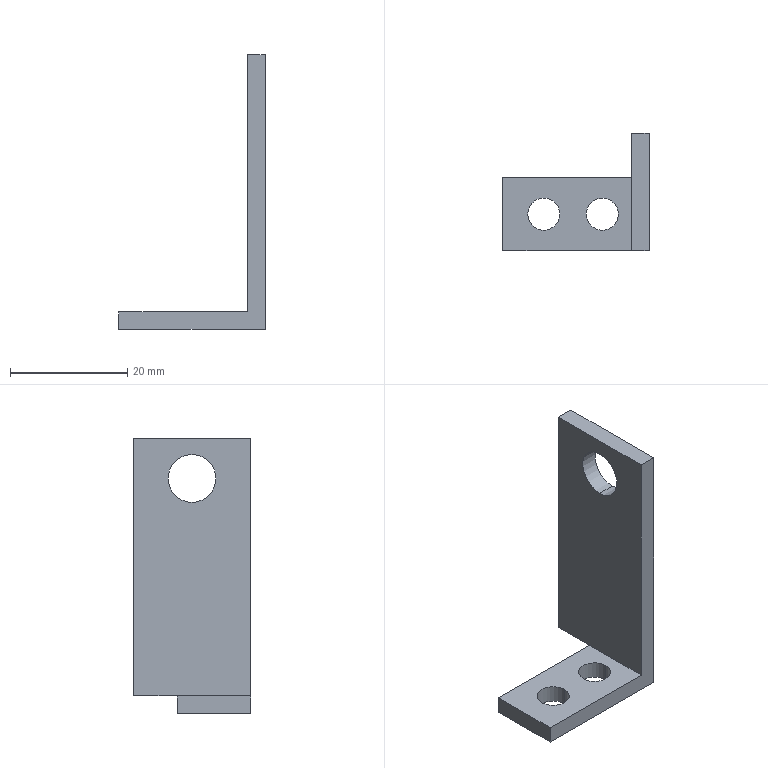Part | 1 solid | 16 faces | box 25 x 20 x 47 mm | volume 3277 mm3 | plane 10 | cylinder 6 | commonest cylinder face diameters 5.5 x4 8.2 x2
STEP:
#1=CARTESIAN_POINT('',(0.,0.,0.));
#2=DIRECTION('',(0.,0.,1.));
#3=DIRECTION('',(1.,0.,0.));
#4=AXIS2_PLACEMENT_3D('',#1,#2,#3);
#5=CARTESIAN_POINT('',(-283.573,173.,-202.474));
#6=VERTEX_POINT('',#5);
#7=CARTESIAN_POINT('',(-283.573,173.,-194.274));
#8=VERTEX_POINT('',#7);
#9=CARTESIAN_POINT('',(-283.573,173.,-198.374));
#10=DIRECTION('',(1.,0.,0.));
#11=DIRECTION('',(0.,0.,-1.));
#12=AXIS2_PLACEMENT_3D('',#9,#10,#11);
#13=CIRCLE('',#12,4.1);
#14=CARTESIAN_POINT('',(-291.041,173.,-198.374));
#15=DIRECTION('',(-1.,0.,0.));
#16=DIRECTION('',(0.,-1.,0.));
#17=AXIS2_PLACEMENT_3D('',#14,#15,#16);
#18=CYLINDRICAL_SURFACE('',#17,4.1);
#19=CARTESIAN_POINT('',(4.712,-7.468));
#20=DIRECTION('',(-1.,0.));
#21=VECTOR('',#20,1.);
#22=LINE('',#19,#21);
#23=(GEOMETRIC_REPRESENTATION_CONTEXT(2)PARAMETRIC_REPRESENTATION_CONTEXT()REPRESENTATION_CONTEXT('',''));
#24=DEFINITIONAL_REPRESENTATION('',(#22),#23);
#25=PCURVE('',#18,#24);
#26=CARTESIAN_POINT('',(-283.573,162.475,-194.374));
#27=DIRECTION('',(1.,0.,0.));
#28=DIRECTION('',(0.,1.,0.));
#29=AXIS2_PLACEMENT_3D('',#26,#27,#28);
#30=PLANE('',#29);
#31=CARTESIAN_POINT('',(10.525,-4.));
#32=DIRECTION('',(0.,-1.));
#33=AXIS2_PLACEMENT_2D('',#31,#32);
#34=CIRCLE('',#33,4.1);
#35=(GEOMETRIC_REPRESENTATION_CONTEXT(2)PARAMETRIC_REPRESENTATION_CONTEXT()REPRESENTATION_CONTEXT('',''));
#36=DEFINITIONAL_REPRESENTATION('',(#34),#35);
#37=PCURVE('',#30,#36);
#38=SURFACE_CURVE('',#13,(#25,#37),.PCURVE_S1.);
#39=EDGE_CURVE('',#6,#8,#38,.T.);
#40=ORIENTED_EDGE('',*,*,#39,.F.);
#41=CARTESIAN_POINT('',(-286.573,173.,-202.474));
#42=VERTEX_POINT('',#41);
#43=CARTESIAN_POINT('',(-283.573,173.,-202.474));
#44=DIRECTION('',(-1.,0.,0.));
#45=VECTOR('',#44,1.);
#46=LINE('',#43,#45);
#47=CARTESIAN_POINT('',(4.712,-7.468));
#48=DIRECTION('',(0.,1.));
#49=VECTOR('',#48,1.);
#50=LINE('',#47,#49);
#51=(GEOMETRIC_REPRESENTATION_CONTEXT(2)PARAMETRIC_REPRESENTATION_CONTEXT()REPRESENTATION_CONTEXT('',''));
#52=DEFINITIONAL_REPRESENTATION('',(#50),#51);
#53=PCURVE('',#18,#52);
#54=CARTESIAN_POINT('',(-291.041,173.,-198.374));
#55=DIRECTION('',(-1.,0.,0.));
#56=DIRECTION('',(0.,1.,0.));
#57=AXIS2_PLACEMENT_3D('',#54,#55,#56);
#58=CYLINDRICAL_SURFACE('',#57,4.1);
#59=CARTESIAN_POINT('',(1.571,-7.468));
#60=DIRECTION('',(0.,1.));
#61=VECTOR('',#60,1.);
#62=LINE('',#59,#61);
#63=(GEOMETRIC_REPRESENTATION_CONTEXT(2)PARAMETRIC_REPRESENTATION_CONTEXT()REPRESENTATION_CONTEXT('',''));
#64=DEFINITIONAL_REPRESENTATION('',(#62),#63);
#65=PCURVE('',#58,#64);
#66=SURFACE_CURVE('',#46,(#53,#65),.PCURVE_S1.);
#67=EDGE_CURVE('',#6,#42,#66,.T.);
#68=ORIENTED_EDGE('',*,*,#67,.T.);
#69=CARTESIAN_POINT('',(-286.573,173.,-194.274));
#70=VERTEX_POINT('',#69);
#71=CARTESIAN_POINT('',(-286.573,173.,-198.374));
#72=DIRECTION('',(-1.,0.,0.));
#73=DIRECTION('',(0.,0.,-1.));
#74=AXIS2_PLACEMENT_3D('',#71,#72,#73);
#75=CIRCLE('',#74,4.1);
#76=CARTESIAN_POINT('',(-1.571,-4.468));
#77=DIRECTION('',(1.,0.));
#78=VECTOR('',#77,1.);
#79=LINE('',#76,#78);
#80=(GEOMETRIC_REPRESENTATION_CONTEXT(2)PARAMETRIC_REPRESENTATION_CONTEXT()REPRESENTATION_CONTEXT('',''));
#81=DEFINITIONAL_REPRESENTATION('',(#79),#80);
#82=PCURVE('',#18,#81);
#83=CARTESIAN_POINT('',(-286.573,162.475,-194.374));
#84=DIRECTION('',(-1.,0.,0.));
#85=DIRECTION('',(0.,-1.,0.));
#86=AXIS2_PLACEMENT_3D('',#83,#84,#85);
#87=PLANE('',#86);
#88=CARTESIAN_POINT('',(-10.525,-4.));
#89=DIRECTION('',(0.,-1.));
#90=AXIS2_PLACEMENT_2D('',#88,#89);
#91=CIRCLE('',#90,4.1);
#92=(GEOMETRIC_REPRESENTATION_CONTEXT(2)PARAMETRIC_REPRESENTATION_CONTEXT()REPRESENTATION_CONTEXT('',''));
#93=DEFINITIONAL_REPRESENTATION('',(#91),#92);
#94=PCURVE('',#87,#93);
#95=SURFACE_CURVE('',#75,(#82,#94),.PCURVE_S1.);
#96=EDGE_CURVE('',#70,#42,#95,.T.);
#97=ORIENTED_EDGE('',*,*,#96,.F.);
#98=CARTESIAN_POINT('',(-283.573,173.,-194.274));
#99=DIRECTION('',(-1.,0.,0.));
#100=VECTOR('',#99,1.);
#101=LINE('',#98,#100);
#102=CARTESIAN_POINT('',(1.571,-7.468));
#103=DIRECTION('',(0.,1.));
#104=VECTOR('',#103,1.);
#105=LINE('',#102,#104);
#106=(GEOMETRIC_REPRESENTATION_CONTEXT(2)PARAMETRIC_REPRESENTATION_CONTEXT()REPRESENTATION_CONTEXT('',''));
#107=DEFINITIONAL_REPRESENTATION('',(#105),#106);
#108=PCURVE('',#18,#107);
#109=CARTESIAN_POINT('',(4.712,-7.468));
#110=DIRECTION('',(0.,1.));
#111=VECTOR('',#110,1.);
#112=LINE('',#109,#111);
#113=(GEOMETRIC_REPRESENTATION_CONTEXT(2)PARAMETRIC_REPRESENTATION_CONTEXT()REPRESENTATION_CONTEXT('',''));
#114=DEFINITIONAL_REPRESENTATION('',(#112),#113);
#115=PCURVE('',#58,#114);
#116=SURFACE_CURVE('',#101,(#108,#115),.PCURVE_S1.);
#117=EDGE_CURVE('',#8,#70,#116,.T.);
#118=ORIENTED_EDGE('',*,*,#117,.F.);
#119=EDGE_LOOP('',(#40,#68,#97,#118));
#120=FACE_BOUND('',#119,.F.);
#121=ADVANCED_FACE('',(#120),#18,.F.);
#122=CARTESIAN_POINT('',(-286.573,183.,-191.55));
#123=VERTEX_POINT('',#122);
#124=CARTESIAN_POINT('',(-286.573,163.,-191.55));
#125=VERTEX_POINT('',#124);
#126=CARTESIAN_POINT('',(-286.573,4.5,-191.55));
#127=DIRECTION('',(0.,-1.,0.));
#128=VECTOR('',#127,1.);
#129=LINE('',#126,#128);
#130=CARTESIAN_POINT('',(157.975,2.824));
#131=DIRECTION('',(1.,0.));
#132=VECTOR('',#131,1.);
#133=LINE('',#130,#132);
#134=(GEOMETRIC_REPRESENTATION_CONTEXT(2)PARAMETRIC_REPRESENTATION_CONTEXT()REPRESENTATION_CONTEXT('',''));
#135=DEFINITIONAL_REPRESENTATION('',(#133),#134);
#136=PCURVE('',#87,#135);
#137=CARTESIAN_POINT('',(-153.465,4.5,-191.55));
#138=DIRECTION('',(0.,0.,1.));
#139=DIRECTION('',(-1.,0.,0.));
#140=AXIS2_PLACEMENT_3D('',#137,#138,#139);
#141=PLANE('',#140);
#142=CARTESIAN_POINT('',(133.108,0.));
#143=DIRECTION('',(0.,1.));
#144=VECTOR('',#143,1.);
#145=LINE('',#142,#144);
#146=(GEOMETRIC_REPRESENTATION_CONTEXT(2)PARAMETRIC_REPRESENTATION_CONTEXT()REPRESENTATION_CONTEXT('',''));
#147=DEFINITIONAL_REPRESENTATION('',(#145),#146);
#148=PCURVE('',#141,#147);
#149=SURFACE_CURVE('',#129,(#136,#148),.PCURVE_S1.);
#150=EDGE_CURVE('',#123,#125,#149,.T.);
#151=ORIENTED_EDGE('',*,*,#150,.F.);
#152=CARTESIAN_POINT('',(-286.573,183.,-235.55));
#153=VERTEX_POINT('',#152);
#154=CARTESIAN_POINT('',(-286.573,183.,-194.374));
#155=DIRECTION('',(0.,0.,-1.));
#156=VECTOR('',#155,1.);
#157=LINE('',#154,#156);
#158=CARTESIAN_POINT('',(-20.525,0.));
#159=DIRECTION('',(0.,-1.));
#160=VECTOR('',#159,1.);
#161=LINE('',#158,#160);
#162=(GEOMETRIC_REPRESENTATION_CONTEXT(2)PARAMETRIC_REPRESENTATION_CONTEXT()REPRESENTATION_CONTEXT('',''));
#163=DEFINITIONAL_REPRESENTATION('',(#161),#162);
#164=PCURVE('',#87,#163);
#165=CARTESIAN_POINT('',(-276.706,183.,-67.661));
#166=DIRECTION('',(0.,1.,0.));
#167=DIRECTION('',(1.,0.,0.));
#168=AXIS2_PLACEMENT_3D('',#165,#166,#167);
#169=PLANE('',#168);
#170=CARTESIAN_POINT('',(-9.868,126.713));
#171=DIRECTION('',(0.,1.));
#172=VECTOR('',#171,1.);
#173=LINE('',#170,#172);
#174=(GEOMETRIC_REPRESENTATION_CONTEXT(2)PARAMETRIC_REPRESENTATION_CONTEXT()REPRESENTATION_CONTEXT('',''));
#175=DEFINITIONAL_REPRESENTATION('',(#173),#174);
#176=PCURVE('',#169,#175);
#177=SURFACE_CURVE('',#157,(#164,#176),.PCURVE_S1.);
#178=EDGE_CURVE('',#123,#153,#177,.T.);
#179=ORIENTED_EDGE('',*,*,#178,.T.);
#180=CARTESIAN_POINT('',(-286.573,175.5,-235.55));
#181=VERTEX_POINT('',#180);
#182=CARTESIAN_POINT('',(-286.573,162.475,-235.55));
#183=DIRECTION('',(0.,-1.,0.));
#184=VECTOR('',#183,1.);
#185=LINE('',#182,#184);
#186=CARTESIAN_POINT('',(0.,-41.176));
#187=DIRECTION('',(1.,0.));
#188=VECTOR('',#187,1.);
#189=LINE('',#186,#188);
#190=(GEOMETRIC_REPRESENTATION_CONTEXT(2)PARAMETRIC_REPRESENTATION_CONTEXT()REPRESENTATION_CONTEXT('',''));
#191=DEFINITIONAL_REPRESENTATION('',(#189),#190);
#192=PCURVE('',#87,#191);
#193=CARTESIAN_POINT('',(-297.573,173.,-235.55));
#194=DIRECTION('',(0.,0.,1.));
#195=DIRECTION('',(-1.,0.,0.));
#196=AXIS2_PLACEMENT_3D('',#193,#194,#195);
#197=PLANE('',#196);
#198=CARTESIAN_POINT('',(-11.,10.525));
#199=DIRECTION('',(0.,1.));
#200=VECTOR('',#199,1.);
#201=LINE('',#198,#200);
#202=(GEOMETRIC_REPRESENTATION_CONTEXT(2)PARAMETRIC_REPRESENTATION_CONTEXT()REPRESENTATION_CONTEXT('',''));
#203=DEFINITIONAL_REPRESENTATION('',(#201),#202);
#204=PCURVE('',#197,#203);
#205=SURFACE_CURVE('',#185,(#192,#204),.PCURVE_S1.);
#206=EDGE_CURVE('',#153,#181,#205,.T.);
#207=ORIENTED_EDGE('',*,*,#206,.T.);
#208=CARTESIAN_POINT('',(-286.573,163.,-235.55));
#209=VERTEX_POINT('',#208);
#210=CARTESIAN_POINT('',(-286.573,162.475,-235.55));
#211=DIRECTION('',(0.,-1.,0.));
#212=VECTOR('',#211,1.);
#213=LINE('',#210,#212);
#214=CARTESIAN_POINT('',(0.,-41.176));
#215=DIRECTION('',(1.,0.));
#216=VECTOR('',#215,1.);
#217=LINE('',#214,#216);
#218=(GEOMETRIC_REPRESENTATION_CONTEXT(2)PARAMETRIC_REPRESENTATION_CONTEXT()REPRESENTATION_CONTEXT('',''));
#219=DEFINITIONAL_REPRESENTATION('',(#217),#218);
#220=PCURVE('',#87,#219);
#221=CARTESIAN_POINT('',(-153.465,4.5,-235.55));
#222=DIRECTION('',(0.,0.,1.));
#223=DIRECTION('',(-1.,0.,0.));
#224=AXIS2_PLACEMENT_3D('',#221,#222,#223);
#225=PLANE('',#224);
#226=CARTESIAN_POINT('',(133.108,-157.975));
#227=DIRECTION('',(0.,1.));
#228=VECTOR('',#227,1.);
#229=LINE('',#226,#228);
#230=(GEOMETRIC_REPRESENTATION_CONTEXT(2)PARAMETRIC_REPRESENTATION_CONTEXT()REPRESENTATION_CONTEXT('',''));
#231=DEFINITIONAL_REPRESENTATION('',(#229),#230);
#232=PCURVE('',#225,#231);
#233=SURFACE_CURVE('',#213,(#220,#232),.PCURVE_S1.);
#234=EDGE_CURVE('',#181,#209,#233,.T.);
#235=ORIENTED_EDGE('',*,*,#234,.T.);
#236=CARTESIAN_POINT('',(-286.573,163.,-194.374));
#237=DIRECTION('',(0.,0.,1.));
#238=VECTOR('',#237,1.);
#239=LINE('',#236,#238);
#240=CARTESIAN_POINT('',(-0.525,0.));
#241=DIRECTION('',(0.,1.));
#242=VECTOR('',#241,1.);
#243=LINE('',#240,#242);
#244=(GEOMETRIC_REPRESENTATION_CONTEXT(2)PARAMETRIC_REPRESENTATION_CONTEXT()REPRESENTATION_CONTEXT('',''));
#245=DEFINITIONAL_REPRESENTATION('',(#243),#244);
#246=PCURVE('',#87,#245);
#247=CARTESIAN_POINT('',(-276.706,163.,-67.661));
#248=DIRECTION('',(0.,1.,0.));
#249=DIRECTION('',(1.,0.,0.));
#250=AXIS2_PLACEMENT_3D('',#247,#248,#249);
#251=PLANE('',#250);
#252=CARTESIAN_POINT('',(-9.868,126.713));
#253=DIRECTION('',(0.,-1.));
#254=VECTOR('',#253,1.);
#255=LINE('',#252,#254);
#256=(GEOMETRIC_REPRESENTATION_CONTEXT(2)PARAMETRIC_REPRESENTATION_CONTEXT()REPRESENTATION_CONTEXT('',''));
#257=DEFINITIONAL_REPRESENTATION('',(#255),#256);
#258=PCURVE('',#251,#257);
#259=SURFACE_CURVE('',#239,(#246,#258),.PCURVE_S1.);
#260=EDGE_CURVE('',#209,#125,#259,.T.);
#261=ORIENTED_EDGE('',*,*,#260,.T.);
#262=EDGE_LOOP('',(#151,#179,#207,#235,#261));
#263=FACE_BOUND('',#262,.T.);
#264=ORIENTED_EDGE('',*,*,#96,.F.);
#265=CARTESIAN_POINT('',(-286.573,173.,-198.374));
#266=DIRECTION('',(-1.,0.,0.));
#267=DIRECTION('',(0.,0.,-1.));
#268=AXIS2_PLACEMENT_3D('',#265,#266,#267);
#269=CIRCLE('',#268,4.1);
#270=CARTESIAN_POINT('',(-10.525,-4.));
#271=DIRECTION('',(0.,-1.));
#272=AXIS2_PLACEMENT_2D('',#270,#271);
#273=CIRCLE('',#272,4.1);
#274=(GEOMETRIC_REPRESENTATION_CONTEXT(2)PARAMETRIC_REPRESENTATION_CONTEXT()REPRESENTATION_CONTEXT('',''));
#275=DEFINITIONAL_REPRESENTATION('',(#273),#274);
#276=PCURVE('',#87,#275);
#277=CARTESIAN_POINT('',(1.571,-4.468));
#278=DIRECTION('',(1.,0.));
#279=VECTOR('',#278,1.);
#280=LINE('',#277,#279);
#281=(GEOMETRIC_REPRESENTATION_CONTEXT(2)PARAMETRIC_REPRESENTATION_CONTEXT()REPRESENTATION_CONTEXT('',''));
#282=DEFINITIONAL_REPRESENTATION('',(#280),#281);
#283=PCURVE('',#58,#282);
#284=SURFACE_CURVE('',#269,(#276,#283),.PCURVE_S1.);
#285=EDGE_CURVE('',#42,#70,#284,.T.);
#286=ORIENTED_EDGE('',*,*,#285,.F.);
#287=EDGE_LOOP('',(#264,#286));
#288=FACE_BOUND('',#287,.T.);
#289=ADVANCED_FACE('',(#263,#288),#87,.T.);
#290=ORIENTED_EDGE('',*,*,#260,.F.);
#291=CARTESIAN_POINT('',(-308.573,163.,-235.55));
#292=VERTEX_POINT('',#291);
#293=CARTESIAN_POINT('',(-276.706,163.,-235.55));
#294=DIRECTION('',(1.,0.,0.));
#295=VECTOR('',#294,1.);
#296=LINE('',#293,#295);
#297=CARTESIAN_POINT('',(0.,167.889));
#298=DIRECTION('',(1.,0.));
#299=VECTOR('',#298,1.);
#300=LINE('',#297,#299);
#301=(GEOMETRIC_REPRESENTATION_CONTEXT(2)PARAMETRIC_REPRESENTATION_CONTEXT()REPRESENTATION_CONTEXT('',''));
#302=DEFINITIONAL_REPRESENTATION('',(#300),#301);
#303=PCURVE('',#251,#302);
#304=CARTESIAN_POINT('',(123.24,-158.5));
#305=DIRECTION('',(-1.,0.));
#306=VECTOR('',#305,1.);
#307=LINE('',#304,#306);
#308=(GEOMETRIC_REPRESENTATION_CONTEXT(2)PARAMETRIC_REPRESENTATION_CONTEXT()REPRESENTATION_CONTEXT('',''));
#309=DEFINITIONAL_REPRESENTATION('',(#307),#308);
#310=PCURVE('',#225,#309);
#311=SURFACE_CURVE('',#296,(#303,#310),.PCURVE_S1.);
#312=EDGE_CURVE('',#292,#209,#311,.T.);
#313=ORIENTED_EDGE('',*,*,#312,.F.);
#314=CARTESIAN_POINT('',(-308.573,163.,-238.55));
#315=VERTEX_POINT('',#314);
#316=CARTESIAN_POINT('',(-308.573,163.,-194.374));
#317=DIRECTION('',(0.,0.,1.));
#318=VECTOR('',#317,1.);
#319=LINE('',#316,#318);
#320=CARTESIAN_POINT('',(-31.868,126.713));
#321=DIRECTION('',(0.,-1.));
#322=VECTOR('',#321,1.);
#323=LINE('',#320,#322);
#324=(GEOMETRIC_REPRESENTATION_CONTEXT(2)PARAMETRIC_REPRESENTATION_CONTEXT()REPRESENTATION_CONTEXT('',''));
#325=DEFINITIONAL_REPRESENTATION('',(#323),#324);
#326=PCURVE('',#251,#325);
#327=CARTESIAN_POINT('',(-308.573,162.475,-194.374));
#328=DIRECTION('',(1.,0.,0.));
#329=DIRECTION('',(0.,1.,0.));
#330=AXIS2_PLACEMENT_3D('',#327,#328,#329);
#331=PLANE('',#330);
#332=CARTESIAN_POINT('',(0.525,0.));
#333=DIRECTION('',(0.,1.));
#334=VECTOR('',#333,1.);
#335=LINE('',#332,#334);
#336=(GEOMETRIC_REPRESENTATION_CONTEXT(2)PARAMETRIC_REPRESENTATION_CONTEXT()REPRESENTATION_CONTEXT('',''));
#337=DEFINITIONAL_REPRESENTATION('',(#335),#336);
#338=PCURVE('',#331,#337);
#339=SURFACE_CURVE('',#319,(#326,#338),.PCURVE_S1.);
#340=EDGE_CURVE('',#315,#292,#339,.T.);
#341=ORIENTED_EDGE('',*,*,#340,.F.);
#342=CARTESIAN_POINT('',(-283.573,163.,-238.55));
#343=VERTEX_POINT('',#342);
#344=CARTESIAN_POINT('',(-153.465,163.,-238.55));
#345=DIRECTION('',(-1.,0.,0.));
#346=VECTOR('',#345,1.);
#347=LINE('',#344,#346);
#348=CARTESIAN_POINT('',(123.24,170.889));
#349=DIRECTION('',(-1.,0.));
#350=VECTOR('',#349,1.);
#351=LINE('',#348,#350);
#352=(GEOMETRIC_REPRESENTATION_CONTEXT(2)PARAMETRIC_REPRESENTATION_CONTEXT()REPRESENTATION_CONTEXT('',''));
#353=DEFINITIONAL_REPRESENTATION('',(#351),#352);
#354=PCURVE('',#251,#353);
#355=CARTESIAN_POINT('',(-153.465,4.5,-238.55));
#356=DIRECTION('',(0.,0.,1.));
#357=DIRECTION('',(-1.,0.,0.));
#358=AXIS2_PLACEMENT_3D('',#355,#356,#357);
#359=PLANE('',#358);
#360=CARTESIAN_POINT('',(0.,-158.5));
#361=DIRECTION('',(1.,0.));
#362=VECTOR('',#361,1.);
#363=LINE('',#360,#362);
#364=(GEOMETRIC_REPRESENTATION_CONTEXT(2)PARAMETRIC_REPRESENTATION_CONTEXT()REPRESENTATION_CONTEXT('',''));
#365=DEFINITIONAL_REPRESENTATION('',(#363),#364);
#366=PCURVE('',#359,#365);
#367=SURFACE_CURVE('',#347,(#354,#366),.PCURVE_S1.);
#368=EDGE_CURVE('',#343,#315,#367,.T.);
#369=ORIENTED_EDGE('',*,*,#368,.F.);
#370=CARTESIAN_POINT('',(-283.573,163.,-191.55));
#371=VERTEX_POINT('',#370);
#372=CARTESIAN_POINT('',(-283.573,163.,-194.374));
#373=DIRECTION('',(0.,0.,-1.));
#374=VECTOR('',#373,1.);
#375=LINE('',#372,#374);
#376=CARTESIAN_POINT('',(-6.868,126.713));
#377=DIRECTION('',(0.,1.));
#378=VECTOR('',#377,1.);
#379=LINE('',#376,#378);
#380=(GEOMETRIC_REPRESENTATION_CONTEXT(2)PARAMETRIC_REPRESENTATION_CONTEXT()REPRESENTATION_CONTEXT('',''));
#381=DEFINITIONAL_REPRESENTATION('',(#379),#380);
#382=PCURVE('',#251,#381);
#383=CARTESIAN_POINT('',(0.525,0.));
#384=DIRECTION('',(0.,-1.));
#385=VECTOR('',#384,1.);
#386=LINE('',#383,#385);
#387=(GEOMETRIC_REPRESENTATION_CONTEXT(2)PARAMETRIC_REPRESENTATION_CONTEXT()REPRESENTATION_CONTEXT('',''));
#388=DEFINITIONAL_REPRESENTATION('',(#386),#387);
#389=PCURVE('',#30,#388);
#390=SURFACE_CURVE('',#375,(#382,#389),.PCURVE_S1.);
#391=EDGE_CURVE('',#371,#343,#390,.T.);
#392=ORIENTED_EDGE('',*,*,#391,.F.);
#393=CARTESIAN_POINT('',(-153.465,163.,-191.55));
#394=DIRECTION('',(1.,0.,0.));
#395=VECTOR('',#394,1.);
#396=LINE('',#393,#395);
#397=CARTESIAN_POINT('',(123.24,123.889));
#398=DIRECTION('',(1.,0.));
#399=VECTOR('',#398,1.);
#400=LINE('',#397,#399);
#401=(GEOMETRIC_REPRESENTATION_CONTEXT(2)PARAMETRIC_REPRESENTATION_CONTEXT()REPRESENTATION_CONTEXT('',''));
#402=DEFINITIONAL_REPRESENTATION('',(#400),#401);
#403=PCURVE('',#251,#402);
#404=CARTESIAN_POINT('',(0.,-158.5));
#405=DIRECTION('',(-1.,0.));
#406=VECTOR('',#405,1.);
#407=LINE('',#404,#406);
#408=(GEOMETRIC_REPRESENTATION_CONTEXT(2)PARAMETRIC_REPRESENTATION_CONTEXT()REPRESENTATION_CONTEXT('',''));
#409=DEFINITIONAL_REPRESENTATION('',(#407),#408);
#410=PCURVE('',#141,#409);
#411=SURFACE_CURVE('',#396,(#403,#410),.PCURVE_S1.);
#412=EDGE_CURVE('',#125,#371,#411,.T.);
#413=ORIENTED_EDGE('',*,*,#412,.F.);
#414=EDGE_LOOP('',(#290,#313,#341,#369,#392,#413));
#415=FACE_BOUND('',#414,.T.);
#416=ADVANCED_FACE('',(#415),#251,.F.);
#417=CARTESIAN_POINT('',(-283.573,183.,-191.55));
#418=VERTEX_POINT('',#417);
#419=CARTESIAN_POINT('',(-283.573,162.475,-191.55));
#420=DIRECTION('',(0.,-1.,0.));
#421=VECTOR('',#420,1.);
#422=LINE('',#419,#421);
#423=CARTESIAN_POINT('',(130.108,-157.975));
#424=DIRECTION('',(0.,1.));
#425=VECTOR('',#424,1.);
#426=LINE('',#423,#425);
#427=(GEOMETRIC_REPRESENTATION_CONTEXT(2)PARAMETRIC_REPRESENTATION_CONTEXT()REPRESENTATION_CONTEXT('',''));
#428=DEFINITIONAL_REPRESENTATION('',(#426),#427);
#429=PCURVE('',#141,#428);
#430=CARTESIAN_POINT('',(0.,2.824));
#431=DIRECTION('',(-1.,0.));
#432=VECTOR('',#431,1.);
#433=LINE('',#430,#432);
#434=(GEOMETRIC_REPRESENTATION_CONTEXT(2)PARAMETRIC_REPRESENTATION_CONTEXT()REPRESENTATION_CONTEXT('',''));
#435=DEFINITIONAL_REPRESENTATION('',(#433),#434);
#436=PCURVE('',#30,#435);
#437=SURFACE_CURVE('',#422,(#429,#436),.PCURVE_S1.);
#438=EDGE_CURVE('',#418,#371,#437,.T.);
#439=ORIENTED_EDGE('',*,*,#438,.F.);
#440=CARTESIAN_POINT('',(-153.465,183.,-191.55));
#441=DIRECTION('',(-1.,0.,0.));
#442=VECTOR('',#441,1.);
#443=LINE('',#440,#442);
#444=CARTESIAN_POINT('',(0.,-178.5));
#445=DIRECTION('',(1.,0.));
#446=VECTOR('',#445,1.);
#447=LINE('',#444,#446);
#448=(GEOMETRIC_REPRESENTATION_CONTEXT(2)PARAMETRIC_REPRESENTATION_CONTEXT()REPRESENTATION_CONTEXT('',''));
#449=DEFINITIONAL_REPRESENTATION('',(#447),#448);
#450=PCURVE('',#141,#449);
#451=CARTESIAN_POINT('',(123.24,123.889));
#452=DIRECTION('',(-1.,0.));
#453=VECTOR('',#452,1.);
#454=LINE('',#451,#453);
#455=(GEOMETRIC_REPRESENTATION_CONTEXT(2)PARAMETRIC_REPRESENTATION_CONTEXT()REPRESENTATION_CONTEXT('',''));
#456=DEFINITIONAL_REPRESENTATION('',(#454),#455);
#457=PCURVE('',#169,#456);
#458=SURFACE_CURVE('',#443,(#450,#457),.PCURVE_S1.);
#459=EDGE_CURVE('',#418,#123,#458,.T.);
#460=ORIENTED_EDGE('',*,*,#459,.T.);
#461=ORIENTED_EDGE('',*,*,#150,.T.);
#462=ORIENTED_EDGE('',*,*,#412,.T.);
#463=EDGE_LOOP('',(#439,#460,#461,#462));
#464=FACE_BOUND('',#463,.T.);
#465=ADVANCED_FACE('',(#464),#141,.T.);
#466=CARTESIAN_POINT('',(-283.573,183.,-235.55));
#467=VERTEX_POINT('',#466);
#468=CARTESIAN_POINT('',(-276.706,183.,-235.55));
#469=DIRECTION('',(1.,0.,0.));
#470=VECTOR('',#469,1.);
#471=LINE('',#468,#470);
#472=CARTESIAN_POINT('',(0.,167.889));
#473=DIRECTION('',(1.,0.));
#474=VECTOR('',#473,1.);
#475=LINE('',#472,#474);
#476=(GEOMETRIC_REPRESENTATION_CONTEXT(2)PARAMETRIC_REPRESENTATION_CONTEXT()REPRESENTATION_CONTEXT('',''));
#477=DEFINITIONAL_REPRESENTATION('',(#475),#476);
#478=PCURVE('',#169,#477);
#479=CARTESIAN_POINT('',(-20.868,-10.));
#480=DIRECTION('',(-1.,0.));
#481=VECTOR('',#480,1.);
#482=LINE('',#479,#481);
#483=(GEOMETRIC_REPRESENTATION_CONTEXT(2)PARAMETRIC_REPRESENTATION_CONTEXT()REPRESENTATION_CONTEXT('',''));
#484=DEFINITIONAL_REPRESENTATION('',(#482),#483);
#485=PCURVE('',#197,#484);
#486=SURFACE_CURVE('',#471,(#478,#485),.PCURVE_S1.);
#487=EDGE_CURVE('',#153,#467,#486,.T.);
#488=ORIENTED_EDGE('',*,*,#487,.F.);
#489=ORIENTED_EDGE('',*,*,#178,.F.);
#490=ORIENTED_EDGE('',*,*,#459,.F.);
#491=CARTESIAN_POINT('',(-283.573,183.,-194.374));
#492=DIRECTION('',(0.,0.,1.));
#493=VECTOR('',#492,1.);
#494=LINE('',#491,#493);
#495=CARTESIAN_POINT('',(-6.868,126.713));
#496=DIRECTION('',(0.,-1.));
#497=VECTOR('',#496,1.);
#498=LINE('',#495,#497);
#499=(GEOMETRIC_REPRESENTATION_CONTEXT(2)PARAMETRIC_REPRESENTATION_CONTEXT()REPRESENTATION_CONTEXT('',''));
#500=DEFINITIONAL_REPRESENTATION('',(#498),#499);
#501=PCURVE('',#169,#500);
#502=CARTESIAN_POINT('',(20.525,0.));
#503=DIRECTION('',(0.,1.));
#504=VECTOR('',#503,1.);
#505=LINE('',#502,#504);
#506=(GEOMETRIC_REPRESENTATION_CONTEXT(2)PARAMETRIC_REPRESENTATION_CONTEXT()REPRESENTATION_CONTEXT('',''));
#507=DEFINITIONAL_REPRESENTATION('',(#505),#506);
#508=PCURVE('',#30,#507);
#509=SURFACE_CURVE('',#494,(#501,#508),.PCURVE_S1.);
#510=EDGE_CURVE('',#467,#418,#509,.T.);
#511=ORIENTED_EDGE('',*,*,#510,.F.);
#512=EDGE_LOOP('',(#488,#489,#490,#511));
#513=FACE_BOUND('',#512,.T.);
#514=ADVANCED_FACE('',(#513),#169,.T.);
#515=CARTESIAN_POINT('',(-283.573,175.5,-235.55));
#516=VERTEX_POINT('',#515);
#517=CARTESIAN_POINT('',(-283.573,162.475,-235.55));
#518=DIRECTION('',(0.,-1.,0.));
#519=VECTOR('',#518,1.);
#520=LINE('',#517,#519);
#521=CARTESIAN_POINT('',(0.,-41.176));
#522=DIRECTION('',(-1.,0.));
#523=VECTOR('',#522,1.);
#524=LINE('',#521,#523);
#525=(GEOMETRIC_REPRESENTATION_CONTEXT(2)PARAMETRIC_REPRESENTATION_CONTEXT()REPRESENTATION_CONTEXT('',''));
#526=DEFINITIONAL_REPRESENTATION('',(#524),#525);
#527=PCURVE('',#30,#526);
#528=CARTESIAN_POINT('',(-14.,10.525));
#529=DIRECTION('',(0.,1.));
#530=VECTOR('',#529,1.);
#531=LINE('',#528,#530);
#532=(GEOMETRIC_REPRESENTATION_CONTEXT(2)PARAMETRIC_REPRESENTATION_CONTEXT()REPRESENTATION_CONTEXT('',''));
#533=DEFINITIONAL_REPRESENTATION('',(#531),#532);
#534=PCURVE('',#197,#533);
#535=SURFACE_CURVE('',#520,(#527,#534),.PCURVE_S1.);
#536=EDGE_CURVE('',#467,#516,#535,.T.);
#537=ORIENTED_EDGE('',*,*,#536,.F.);
#538=ORIENTED_EDGE('',*,*,#510,.T.);
#539=ORIENTED_EDGE('',*,*,#438,.T.);
#540=ORIENTED_EDGE('',*,*,#391,.T.);
#541=CARTESIAN_POINT('',(-283.573,175.5,-238.55));
#542=VERTEX_POINT('',#541);
#543=CARTESIAN_POINT('',(-283.573,162.475,-238.55));
#544=DIRECTION('',(0.,-1.,0.));
#545=VECTOR('',#544,1.);
#546=LINE('',#543,#545);
#547=CARTESIAN_POINT('',(0.,-44.176));
#548=DIRECTION('',(-1.,0.));
#549=VECTOR('',#548,1.);
#550=LINE('',#547,#549);
#551=(GEOMETRIC_REPRESENTATION_CONTEXT(2)PARAMETRIC_REPRESENTATION_CONTEXT()REPRESENTATION_CONTEXT('',''));
#552=DEFINITIONAL_REPRESENTATION('',(#550),#551);
#553=PCURVE('',#30,#552);
#554=CARTESIAN_POINT('',(130.108,-157.975));
#555=DIRECTION('',(0.,1.));
#556=VECTOR('',#555,1.);
#557=LINE('',#554,#556);
#558=(GEOMETRIC_REPRESENTATION_CONTEXT(2)PARAMETRIC_REPRESENTATION_CONTEXT()REPRESENTATION_CONTEXT('',''));
#559=DEFINITIONAL_REPRESENTATION('',(#557),#558);
#560=PCURVE('',#359,#559);
#561=SURFACE_CURVE('',#546,(#553,#560),.PCURVE_S1.);
#562=EDGE_CURVE('',#542,#343,#561,.T.);
#563=ORIENTED_EDGE('',*,*,#562,.F.);
#564=CARTESIAN_POINT('',(-283.573,175.5,-194.374));
#565=DIRECTION('',(0.,0.,1.));
#566=VECTOR('',#565,1.);
#567=LINE('',#564,#566);
#568=CARTESIAN_POINT('',(13.025,0.));
#569=DIRECTION('',(0.,1.));
#570=VECTOR('',#569,1.);
#571=LINE('',#568,#570);
#572=(GEOMETRIC_REPRESENTATION_CONTEXT(2)PARAMETRIC_REPRESENTATION_CONTEXT()REPRESENTATION_CONTEXT('',''));
#573=DEFINITIONAL_REPRESENTATION('',(#571),#572);
#574=PCURVE('',#30,#573);
#575=CARTESIAN_POINT('',(-276.706,175.5,-67.661));
#576=DIRECTION('',(0.,1.,0.));
#577=DIRECTION('',(1.,0.,0.));
#578=AXIS2_PLACEMENT_3D('',#575,#576,#577);
#579=PLANE('',#578);
#580=CARTESIAN_POINT('',(-6.868,126.713));
#581=DIRECTION('',(0.,-1.));
#582=VECTOR('',#581,1.);
#583=LINE('',#580,#582);
#584=(GEOMETRIC_REPRESENTATION_CONTEXT(2)PARAMETRIC_REPRESENTATION_CONTEXT()REPRESENTATION_CONTEXT('',''));
#585=DEFINITIONAL_REPRESENTATION('',(#583),#584);
#586=PCURVE('',#579,#585);
#587=SURFACE_CURVE('',#567,(#574,#586),.PCURVE_S1.);
#588=EDGE_CURVE('',#542,#516,#587,.T.);
#589=ORIENTED_EDGE('',*,*,#588,.T.);
#590=EDGE_LOOP('',(#537,#538,#539,#540,#563,#589));
#591=FACE_BOUND('',#590,.T.);
#592=CARTESIAN_POINT('',(-283.573,173.,-198.374));
#593=DIRECTION('',(1.,0.,0.));
#594=DIRECTION('',(0.,0.,-1.));
#595=AXIS2_PLACEMENT_3D('',#592,#593,#594);
#596=CIRCLE('',#595,4.1);
#597=CARTESIAN_POINT('',(10.525,-4.));
#598=DIRECTION('',(0.,-1.));
#599=AXIS2_PLACEMENT_2D('',#597,#598);
#600=CIRCLE('',#599,4.1);
#601=(GEOMETRIC_REPRESENTATION_CONTEXT(2)PARAMETRIC_REPRESENTATION_CONTEXT()REPRESENTATION_CONTEXT('',''));
#602=DEFINITIONAL_REPRESENTATION('',(#600),#601);
#603=PCURVE('',#30,#602);
#604=CARTESIAN_POINT('',(7.854,-7.468));
#605=DIRECTION('',(-1.,0.));
#606=VECTOR('',#605,1.);
#607=LINE('',#604,#606);
#608=(GEOMETRIC_REPRESENTATION_CONTEXT(2)PARAMETRIC_REPRESENTATION_CONTEXT()REPRESENTATION_CONTEXT('',''));
#609=DEFINITIONAL_REPRESENTATION('',(#607),#608);
#610=PCURVE('',#58,#609);
#611=SURFACE_CURVE('',#596,(#603,#610),.PCURVE_S1.);
#612=EDGE_CURVE('',#8,#6,#611,.T.);
#613=ORIENTED_EDGE('',*,*,#612,.F.);
#614=ORIENTED_EDGE('',*,*,#39,.F.);
#615=EDGE_LOOP('',(#613,#614));
#616=FACE_BOUND('',#615,.T.);
#617=ADVANCED_FACE('',(#591,#616),#30,.T.);
#618=CARTESIAN_POINT('',(-308.573,175.5,-235.55));
#619=VERTEX_POINT('',#618);
#620=CARTESIAN_POINT('',(-308.573,175.5,-238.55));
#621=VERTEX_POINT('',#620);
#622=CARTESIAN_POINT('',(-308.573,175.5,-194.374));
#623=DIRECTION('',(0.,0.,-1.));
#624=VECTOR('',#623,1.);
#625=LINE('',#622,#624);
#626=CARTESIAN_POINT('',(-31.868,126.713));
#627=DIRECTION('',(0.,1.));
#628=VECTOR('',#627,1.);
#629=LINE('',#626,#628);
#630=(GEOMETRIC_REPRESENTATION_CONTEXT(2)PARAMETRIC_REPRESENTATION_CONTEXT()REPRESENTATION_CONTEXT('',''));
#631=DEFINITIONAL_REPRESENTATION('',(#629),#630);
#632=PCURVE('',#579,#631);
#633=CARTESIAN_POINT('',(13.025,0.));
#634=DIRECTION('',(0.,-1.));
#635=VECTOR('',#634,1.);
#636=LINE('',#633,#635);
#637=(GEOMETRIC_REPRESENTATION_CONTEXT(2)PARAMETRIC_REPRESENTATION_CONTEXT()REPRESENTATION_CONTEXT('',''));
#638=DEFINITIONAL_REPRESENTATION('',(#636),#637);
#639=PCURVE('',#331,#638);
#640=SURFACE_CURVE('',#625,(#632,#639),.PCURVE_S1.);
#641=EDGE_CURVE('',#619,#621,#640,.T.);
#642=ORIENTED_EDGE('',*,*,#641,.F.);
#643=CARTESIAN_POINT('',(-153.465,175.5,-235.55));
#644=DIRECTION('',(-1.,0.,0.));
#645=VECTOR('',#644,1.);
#646=LINE('',#643,#645);
#647=CARTESIAN_POINT('',(123.24,167.889));
#648=DIRECTION('',(-1.,0.));
#649=VECTOR('',#648,1.);
#650=LINE('',#647,#649);
#651=(GEOMETRIC_REPRESENTATION_CONTEXT(2)PARAMETRIC_REPRESENTATION_CONTEXT()REPRESENTATION_CONTEXT('',''));
#652=DEFINITIONAL_REPRESENTATION('',(#650),#651);
#653=PCURVE('',#579,#652);
#654=CARTESIAN_POINT('',(0.,-171.));
#655=DIRECTION('',(1.,0.));
#656=VECTOR('',#655,1.);
#657=LINE('',#654,#656);
#658=(GEOMETRIC_REPRESENTATION_CONTEXT(2)PARAMETRIC_REPRESENTATION_CONTEXT()REPRESENTATION_CONTEXT('',''));
#659=DEFINITIONAL_REPRESENTATION('',(#657),#658);
#660=PCURVE('',#225,#659);
#661=SURFACE_CURVE('',#646,(#653,#660),.PCURVE_S1.);
#662=EDGE_CURVE('',#181,#619,#661,.T.);
#663=ORIENTED_EDGE('',*,*,#662,.F.);
#664=CARTESIAN_POINT('',(-153.465,175.5,-235.55));
#665=DIRECTION('',(-1.,0.,0.));
#666=VECTOR('',#665,1.);
#667=LINE('',#664,#666);
#668=CARTESIAN_POINT('',(123.24,167.889));
#669=DIRECTION('',(-1.,0.));
#670=VECTOR('',#669,1.);
#671=LINE('',#668,#670);
#672=(GEOMETRIC_REPRESENTATION_CONTEXT(2)PARAMETRIC_REPRESENTATION_CONTEXT()REPRESENTATION_CONTEXT('',''));
#673=DEFINITIONAL_REPRESENTATION('',(#671),#672);
#674=PCURVE('',#579,#673);
#675=CARTESIAN_POINT('',(-144.108,-2.5));
#676=DIRECTION('',(1.,0.));
#677=VECTOR('',#676,1.);
#678=LINE('',#675,#677);
#679=(GEOMETRIC_REPRESENTATION_CONTEXT(2)PARAMETRIC_REPRESENTATION_CONTEXT()REPRESENTATION_CONTEXT('',''));
#680=DEFINITIONAL_REPRESENTATION('',(#678),#679);
#681=PCURVE('',#197,#680);
#682=SURFACE_CURVE('',#667,(#674,#681),.PCURVE_S1.);
#683=EDGE_CURVE('',#516,#181,#682,.T.);
#684=ORIENTED_EDGE('',*,*,#683,.F.);
#685=ORIENTED_EDGE('',*,*,#588,.F.);
#686=CARTESIAN_POINT('',(-153.465,175.5,-238.55));
#687=DIRECTION('',(1.,0.,0.));
#688=VECTOR('',#687,1.);
#689=LINE('',#686,#688);
#690=CARTESIAN_POINT('',(123.24,170.889));
#691=DIRECTION('',(1.,0.));
#692=VECTOR('',#691,1.);
#693=LINE('',#690,#692);
#694=(GEOMETRIC_REPRESENTATION_CONTEXT(2)PARAMETRIC_REPRESENTATION_CONTEXT()REPRESENTATION_CONTEXT('',''));
#695=DEFINITIONAL_REPRESENTATION('',(#693),#694);
#696=PCURVE('',#579,#695);
#697=CARTESIAN_POINT('',(0.,-171.));
#698=DIRECTION('',(-1.,0.));
#699=VECTOR('',#698,1.);
#700=LINE('',#697,#699);
#701=(GEOMETRIC_REPRESENTATION_CONTEXT(2)PARAMETRIC_REPRESENTATION_CONTEXT()REPRESENTATION_CONTEXT('',''));
#702=DEFINITIONAL_REPRESENTATION('',(#700),#701);
#703=PCURVE('',#359,#702);
#704=SURFACE_CURVE('',#689,(#696,#703),.PCURVE_S1.);
#705=EDGE_CURVE('',#621,#542,#704,.T.);
#706=ORIENTED_EDGE('',*,*,#705,.F.);
#707=EDGE_LOOP('',(#642,#663,#684,#685,#706));
#708=FACE_BOUND('',#707,.T.);
#709=ADVANCED_FACE('',(#708),#579,.T.);
#710=CARTESIAN_POINT('',(-298.823,169.25,-238.55));
#711=VERTEX_POINT('',#710);
#712=CARTESIAN_POINT('',(-304.323,169.25,-238.55));
#713=VERTEX_POINT('',#712);
#714=CARTESIAN_POINT('',(-301.573,169.25,-238.55));
#715=DIRECTION('',(0.,0.,1.));
#716=DIRECTION('',(1.,0.,0.));
#717=AXIS2_PLACEMENT_3D('',#714,#715,#716);
#718=CIRCLE('',#717,2.75);
#719=CARTESIAN_POINT('',(148.108,-164.75));
#720=DIRECTION('',(-1.,0.));
#721=AXIS2_PLACEMENT_2D('',#719,#720);
#722=CIRCLE('',#721,2.75);
#723=(GEOMETRIC_REPRESENTATION_CONTEXT(2)PARAMETRIC_REPRESENTATION_CONTEXT()REPRESENTATION_CONTEXT('',''));
#724=DEFINITIONAL_REPRESENTATION('',(#722),#723);
#725=PCURVE('',#359,#724);
#726=CARTESIAN_POINT('',(-301.573,169.25,-235.55));
#727=DIRECTION('',(0.,0.,-1.));
#728=DIRECTION('',(0.,-1.,0.));
#729=AXIS2_PLACEMENT_3D('',#726,#727,#728);
#730=CYLINDRICAL_SURFACE('',#729,2.75);
#731=CARTESIAN_POINT('',(4.712,3.));
#732=DIRECTION('',(-1.,0.));
#733=VECTOR('',#732,1.);
#734=LINE('',#731,#733);
#735=(GEOMETRIC_REPRESENTATION_CONTEXT(2)PARAMETRIC_REPRESENTATION_CONTEXT()REPRESENTATION_CONTEXT('',''));
#736=DEFINITIONAL_REPRESENTATION('',(#734),#735);
#737=PCURVE('',#730,#736);
#738=SURFACE_CURVE('',#718,(#725,#737),.PCURVE_S1.);
#739=EDGE_CURVE('',#711,#713,#738,.T.);
#740=ORIENTED_EDGE('',*,*,#739,.T.);
#741=CARTESIAN_POINT('',(-301.573,169.25,-238.55));
#742=DIRECTION('',(0.,0.,1.));
#743=DIRECTION('',(1.,0.,0.));
#744=AXIS2_PLACEMENT_3D('',#741,#742,#743);
#745=CIRCLE('',#744,2.75);
#746=CARTESIAN_POINT('',(148.108,-164.75));
#747=DIRECTION('',(-1.,0.));
#748=AXIS2_PLACEMENT_2D('',#746,#747);
#749=CIRCLE('',#748,2.75);
#750=(GEOMETRIC_REPRESENTATION_CONTEXT(2)PARAMETRIC_REPRESENTATION_CONTEXT()REPRESENTATION_CONTEXT('',''));
#751=DEFINITIONAL_REPRESENTATION('',(#749),#750);
#752=PCURVE('',#359,#751);
#753=CARTESIAN_POINT('',(-301.573,169.25,-235.55));
#754=DIRECTION('',(0.,0.,-1.));
#755=DIRECTION('',(0.,1.,0.));
#756=AXIS2_PLACEMENT_3D('',#753,#754,#755);
#757=CYLINDRICAL_SURFACE('',#756,2.75);
#758=CARTESIAN_POINT('',(7.854,3.));
#759=DIRECTION('',(-1.,0.));
#760=VECTOR('',#759,1.);
#761=LINE('',#758,#760);
#762=(GEOMETRIC_REPRESENTATION_CONTEXT(2)PARAMETRIC_REPRESENTATION_CONTEXT()REPRESENTATION_CONTEXT('',''));
#763=DEFINITIONAL_REPRESENTATION('',(#761),#762);
#764=PCURVE('',#757,#763);
#765=SURFACE_CURVE('',#745,(#752,#764),.PCURVE_S1.);
#766=EDGE_CURVE('',#713,#711,#765,.T.);
#767=ORIENTED_EDGE('',*,*,#766,.T.);
#768=EDGE_LOOP('',(#740,#767));
#769=FACE_BOUND('',#768,.T.);
#770=CARTESIAN_POINT('',(-288.823,169.25,-238.55));
#771=VERTEX_POINT('',#770);
#772=CARTESIAN_POINT('',(-294.323,169.25,-238.55));
#773=VERTEX_POINT('',#772);
#774=CARTESIAN_POINT('',(-291.573,169.25,-238.55));
#775=DIRECTION('',(0.,0.,1.));
#776=DIRECTION('',(1.,0.,0.));
#777=AXIS2_PLACEMENT_3D('',#774,#775,#776);
#778=CIRCLE('',#777,2.75);
#779=CARTESIAN_POINT('',(138.108,-164.75));
#780=DIRECTION('',(-1.,0.));
#781=AXIS2_PLACEMENT_2D('',#779,#780);
#782=CIRCLE('',#781,2.75);
#783=(GEOMETRIC_REPRESENTATION_CONTEXT(2)PARAMETRIC_REPRESENTATION_CONTEXT()REPRESENTATION_CONTEXT('',''));
#784=DEFINITIONAL_REPRESENTATION('',(#782),#783);
#785=PCURVE('',#359,#784);
#786=CARTESIAN_POINT('',(-291.573,169.25,-235.55));
#787=DIRECTION('',(0.,0.,-1.));
#788=DIRECTION('',(0.,-1.,0.));
#789=AXIS2_PLACEMENT_3D('',#786,#787,#788);
#790=CYLINDRICAL_SURFACE('',#789,2.75);
#791=CARTESIAN_POINT('',(4.712,3.));
#792=DIRECTION('',(-1.,0.));
#793=VECTOR('',#792,1.);
#794=LINE('',#791,#793);
#795=(GEOMETRIC_REPRESENTATION_CONTEXT(2)PARAMETRIC_REPRESENTATION_CONTEXT()REPRESENTATION_CONTEXT('',''));
#796=DEFINITIONAL_REPRESENTATION('',(#794),#795);
#797=PCURVE('',#790,#796);
#798=SURFACE_CURVE('',#778,(#785,#797),.PCURVE_S1.);
#799=EDGE_CURVE('',#771,#773,#798,.T.);
#800=ORIENTED_EDGE('',*,*,#799,.T.);
#801=CARTESIAN_POINT('',(-291.573,169.25,-238.55));
#802=DIRECTION('',(0.,0.,1.));
#803=DIRECTION('',(1.,0.,0.));
#804=AXIS2_PLACEMENT_3D('',#801,#802,#803);
#805=CIRCLE('',#804,2.75);
#806=CARTESIAN_POINT('',(138.108,-164.75));
#807=DIRECTION('',(-1.,0.));
#808=AXIS2_PLACEMENT_2D('',#806,#807);
#809=CIRCLE('',#808,2.75);
#810=(GEOMETRIC_REPRESENTATION_CONTEXT(2)PARAMETRIC_REPRESENTATION_CONTEXT()REPRESENTATION_CONTEXT('',''));
#811=DEFINITIONAL_REPRESENTATION('',(#809),#810);
#812=PCURVE('',#359,#811);
#813=CARTESIAN_POINT('',(-291.573,169.25,-235.55));
#814=DIRECTION('',(0.,0.,-1.));
#815=DIRECTION('',(0.,1.,0.));
#816=AXIS2_PLACEMENT_3D('',#813,#814,#815);
#817=CYLINDRICAL_SURFACE('',#816,2.75);
#818=CARTESIAN_POINT('',(7.854,3.));
#819=DIRECTION('',(-1.,0.));
#820=VECTOR('',#819,1.);
#821=LINE('',#818,#820);
#822=(GEOMETRIC_REPRESENTATION_CONTEXT(2)PARAMETRIC_REPRESENTATION_CONTEXT()REPRESENTATION_CONTEXT('',''));
#823=DEFINITIONAL_REPRESENTATION('',(#821),#822);
#824=PCURVE('',#817,#823);
#825=SURFACE_CURVE('',#805,(#812,#824),.PCURVE_S1.);
#826=EDGE_CURVE('',#773,#771,#825,.T.);
#827=ORIENTED_EDGE('',*,*,#826,.T.);
#828=EDGE_LOOP('',(#800,#827));
#829=FACE_BOUND('',#828,.T.);
#830=CARTESIAN_POINT('',(-308.573,4.5,-238.55));
#831=DIRECTION('',(0.,-1.,0.));
#832=VECTOR('',#831,1.);
#833=LINE('',#830,#832);
#834=CARTESIAN_POINT('',(155.108,0.));
#835=DIRECTION('',(0.,1.));
#836=VECTOR('',#835,1.);
#837=LINE('',#834,#836);
#838=(GEOMETRIC_REPRESENTATION_CONTEXT(2)PARAMETRIC_REPRESENTATION_CONTEXT()REPRESENTATION_CONTEXT('',''));
#839=DEFINITIONAL_REPRESENTATION('',(#837),#838);
#840=PCURVE('',#359,#839);
#841=CARTESIAN_POINT('',(-157.975,-44.176));
#842=DIRECTION('',(-1.,0.));
#843=VECTOR('',#842,1.);
#844=LINE('',#841,#843);
#845=(GEOMETRIC_REPRESENTATION_CONTEXT(2)PARAMETRIC_REPRESENTATION_CONTEXT()REPRESENTATION_CONTEXT('',''));
#846=DEFINITIONAL_REPRESENTATION('',(#844),#845);
#847=PCURVE('',#331,#846);
#848=SURFACE_CURVE('',#833,(#840,#847),.PCURVE_S1.);
#849=EDGE_CURVE('',#621,#315,#848,.T.);
#850=ORIENTED_EDGE('',*,*,#849,.F.);
#851=ORIENTED_EDGE('',*,*,#705,.T.);
#852=ORIENTED_EDGE('',*,*,#562,.T.);
#853=ORIENTED_EDGE('',*,*,#368,.T.);
#854=EDGE_LOOP('',(#850,#851,#852,#853));
#855=FACE_BOUND('',#854,.T.);
#856=ADVANCED_FACE('',(#769,#829,#855),#359,.F.);
#857=CARTESIAN_POINT('',(-308.573,162.475,-235.55));
#858=DIRECTION('',(0.,-1.,0.));
#859=VECTOR('',#858,1.);
#860=LINE('',#857,#859);
#861=CARTESIAN_POINT('',(0.,-41.176));
#862=DIRECTION('',(-1.,0.));
#863=VECTOR('',#862,1.);
#864=LINE('',#861,#863);
#865=(GEOMETRIC_REPRESENTATION_CONTEXT(2)PARAMETRIC_REPRESENTATION_CONTEXT()REPRESENTATION_CONTEXT('',''));
#866=DEFINITIONAL_REPRESENTATION('',(#864),#865);
#867=PCURVE('',#331,#866);
#868=CARTESIAN_POINT('',(155.108,-157.975));
#869=DIRECTION('',(0.,1.));
#870=VECTOR('',#869,1.);
#871=LINE('',#868,#870);
#872=(GEOMETRIC_REPRESENTATION_CONTEXT(2)PARAMETRIC_REPRESENTATION_CONTEXT()REPRESENTATION_CONTEXT('',''));
#873=DEFINITIONAL_REPRESENTATION('',(#871),#872);
#874=PCURVE('',#225,#873);
#875=SURFACE_CURVE('',#860,(#867,#874),.PCURVE_S1.);
#876=EDGE_CURVE('',#619,#292,#875,.T.);
#877=ORIENTED_EDGE('',*,*,#876,.F.);
#878=ORIENTED_EDGE('',*,*,#641,.T.);
#879=ORIENTED_EDGE('',*,*,#849,.T.);
#880=ORIENTED_EDGE('',*,*,#340,.T.);
#881=EDGE_LOOP('',(#877,#878,#879,#880));
#882=FACE_BOUND('',#881,.T.);
#883=ADVANCED_FACE('',(#882),#331,.F.);
#884=CARTESIAN_POINT('',(-294.323,169.25,-235.55));
#885=VERTEX_POINT('',#884);
#886=CARTESIAN_POINT('',(-288.823,169.25,-235.55));
#887=VERTEX_POINT('',#886);
#888=CARTESIAN_POINT('',(-291.573,169.25,-235.55));
#889=DIRECTION('',(0.,0.,1.));
#890=DIRECTION('',(1.,0.,0.));
#891=AXIS2_PLACEMENT_3D('',#888,#889,#890);
#892=CIRCLE('',#891,2.75);
#893=CARTESIAN_POINT('',(138.108,-164.75));
#894=DIRECTION('',(-1.,0.));
#895=AXIS2_PLACEMENT_2D('',#893,#894);
#896=CIRCLE('',#895,2.75);
#897=(GEOMETRIC_REPRESENTATION_CONTEXT(2)PARAMETRIC_REPRESENTATION_CONTEXT()REPRESENTATION_CONTEXT('',''));
#898=DEFINITIONAL_REPRESENTATION('',(#896),#897);
#899=PCURVE('',#225,#898);
#900=CARTESIAN_POINT('',(7.854,0.));
#901=DIRECTION('',(-1.,0.));
#902=VECTOR('',#901,1.);
#903=LINE('',#900,#902);
#904=(GEOMETRIC_REPRESENTATION_CONTEXT(2)PARAMETRIC_REPRESENTATION_CONTEXT()REPRESENTATION_CONTEXT('',''));
#905=DEFINITIONAL_REPRESENTATION('',(#903),#904);
#906=PCURVE('',#817,#905);
#907=SURFACE_CURVE('',#892,(#899,#906),.PCURVE_S1.);
#908=EDGE_CURVE('',#885,#887,#907,.T.);
#909=ORIENTED_EDGE('',*,*,#908,.F.);
#910=CARTESIAN_POINT('',(-291.573,169.25,-235.55));
#911=DIRECTION('',(0.,0.,1.));
#912=DIRECTION('',(1.,0.,0.));
#913=AXIS2_PLACEMENT_3D('',#910,#911,#912);
#914=CIRCLE('',#913,2.75);
#915=CARTESIAN_POINT('',(138.108,-164.75));
#916=DIRECTION('',(-1.,0.));
#917=AXIS2_PLACEMENT_2D('',#915,#916);
#918=CIRCLE('',#917,2.75);
#919=(GEOMETRIC_REPRESENTATION_CONTEXT(2)PARAMETRIC_REPRESENTATION_CONTEXT()REPRESENTATION_CONTEXT('',''));
#920=DEFINITIONAL_REPRESENTATION('',(#918),#919);
#921=PCURVE('',#225,#920);
#922=CARTESIAN_POINT('',(4.712,0.));
#923=DIRECTION('',(-1.,0.));
#924=VECTOR('',#923,1.);
#925=LINE('',#922,#924);
#926=(GEOMETRIC_REPRESENTATION_CONTEXT(2)PARAMETRIC_REPRESENTATION_CONTEXT()REPRESENTATION_CONTEXT('',''));
#927=DEFINITIONAL_REPRESENTATION('',(#925),#926);
#928=PCURVE('',#790,#927);
#929=SURFACE_CURVE('',#914,(#921,#928),.PCURVE_S1.);
#930=EDGE_CURVE('',#887,#885,#929,.T.);
#931=ORIENTED_EDGE('',*,*,#930,.F.);
#932=EDGE_LOOP('',(#909,#931));
#933=FACE_BOUND('',#932,.T.);
#934=CARTESIAN_POINT('',(-298.823,169.25,-235.55));
#935=VERTEX_POINT('',#934);
#936=CARTESIAN_POINT('',(-304.323,169.25,-235.55));
#937=VERTEX_POINT('',#936);
#938=CARTESIAN_POINT('',(-301.573,169.25,-235.55));
#939=DIRECTION('',(0.,0.,-1.));
#940=DIRECTION('',(1.,0.,0.));
#941=AXIS2_PLACEMENT_3D('',#938,#939,#940);
#942=CIRCLE('',#941,2.75);
#943=CARTESIAN_POINT('',(145.358,-164.75));
#944=CARTESIAN_POINT('',(145.358,-159.987));
#945=CARTESIAN_POINT('',(149.483,-162.368));
#946=CARTESIAN_POINT('',(153.608,-164.75));
#947=CARTESIAN_POINT('',(149.483,-167.132));
#948=CARTESIAN_POINT('',(145.358,-169.513));
#949=CARTESIAN_POINT('',(145.358,-164.75));
#950=(BOUNDED_CURVE()B_SPLINE_CURVE(2,(#943,#944,#945,#946,#947,#948,#949),.UNSPECIFIED.,.T.,.F.)B_SPLINE_CURVE_WITH_KNOTS((1,2,2,2,2,1),(-2.094,0.,2.094,4.189,6.283,8.378),.UNSPECIFIED.)CURVE()GEOMETRIC_REPRESENTATION_ITEM()RATIONAL_B_SPLINE_CURVE((1.,0.5,1.,0.5,1.,0.5,1.))REPRESENTATION_ITEM(''));
#951=(GEOMETRIC_REPRESENTATION_CONTEXT(2)PARAMETRIC_REPRESENTATION_CONTEXT()REPRESENTATION_CONTEXT('',''));
#952=DEFINITIONAL_REPRESENTATION('',(#950),#951);
#953=PCURVE('',#225,#952);
#954=CARTESIAN_POINT('',(1.571,0.));
#955=DIRECTION('',(1.,0.));
#956=VECTOR('',#955,1.);
#957=LINE('',#954,#956);
#958=(GEOMETRIC_REPRESENTATION_CONTEXT(2)PARAMETRIC_REPRESENTATION_CONTEXT()REPRESENTATION_CONTEXT('',''));
#959=DEFINITIONAL_REPRESENTATION('',(#957),#958);
#960=PCURVE('',#757,#959);
#961=SURFACE_CURVE('',#942,(#953,#960),.PCURVE_S1.);
#962=EDGE_CURVE('',#935,#937,#961,.T.);
#963=ORIENTED_EDGE('',*,*,#962,.T.);
#964=CARTESIAN_POINT('',(-301.573,169.25,-235.55));
#965=DIRECTION('',(0.,0.,-1.));
#966=DIRECTION('',(1.,0.,0.));
#967=AXIS2_PLACEMENT_3D('',#964,#965,#966);
#968=CIRCLE('',#967,2.75);
#969=CARTESIAN_POINT('',(145.358,-164.75));
#970=CARTESIAN_POINT('',(145.358,-159.987));
#971=CARTESIAN_POINT('',(149.483,-162.368));
#972=CARTESIAN_POINT('',(153.608,-164.75));
#973=CARTESIAN_POINT('',(149.483,-167.132));
#974=CARTESIAN_POINT('',(145.358,-169.513));
#975=CARTESIAN_POINT('',(145.358,-164.75));
#976=(BOUNDED_CURVE()B_SPLINE_CURVE(2,(#969,#970,#971,#972,#973,#974,#975),.UNSPECIFIED.,.T.,.F.)B_SPLINE_CURVE_WITH_KNOTS((1,2,2,2,2,1),(-2.094,0.,2.094,4.189,6.283,8.378),.UNSPECIFIED.)CURVE()GEOMETRIC_REPRESENTATION_ITEM()RATIONAL_B_SPLINE_CURVE((1.,0.5,1.,0.5,1.,0.5,1.))REPRESENTATION_ITEM(''));
#977=(GEOMETRIC_REPRESENTATION_CONTEXT(2)PARAMETRIC_REPRESENTATION_CONTEXT()REPRESENTATION_CONTEXT('',''));
#978=DEFINITIONAL_REPRESENTATION('',(#976),#977);
#979=PCURVE('',#225,#978);
#980=CARTESIAN_POINT('',(-1.571,0.));
#981=DIRECTION('',(1.,0.));
#982=VECTOR('',#981,1.);
#983=LINE('',#980,#982);
#984=(GEOMETRIC_REPRESENTATION_CONTEXT(2)PARAMETRIC_REPRESENTATION_CONTEXT()REPRESENTATION_CONTEXT('',''));
#985=DEFINITIONAL_REPRESENTATION('',(#983),#984);
#986=PCURVE('',#730,#985);
#987=SURFACE_CURVE('',#968,(#979,#986),.PCURVE_S1.);
#988=EDGE_CURVE('',#937,#935,#987,.T.);
#989=ORIENTED_EDGE('',*,*,#988,.T.);
#990=EDGE_LOOP('',(#963,#989));
#991=FACE_BOUND('',#990,.T.);
#992=ORIENTED_EDGE('',*,*,#234,.F.);
#993=ORIENTED_EDGE('',*,*,#662,.T.);
#994=ORIENTED_EDGE('',*,*,#876,.T.);
#995=ORIENTED_EDGE('',*,*,#312,.T.);
#996=EDGE_LOOP('',(#992,#993,#994,#995));
#997=FACE_BOUND('',#996,.T.);
#998=ADVANCED_FACE('',(#933,#991,#997),#225,.T.);
#999=ORIENTED_EDGE('',*,*,#988,.T.);
#1000=CARTESIAN_POINT('',(-298.823,169.25,-235.55));
#1001=DIRECTION('',(0.,0.,-1.));
#1002=VECTOR('',#1001,1.);
#1003=LINE('',#1000,#1002);
#1004=CARTESIAN_POINT('',(4.712,0.));
#1005=DIRECTION('',(0.,1.));
#1006=VECTOR('',#1005,1.);
#1007=LINE('',#1004,#1006);
#1008=(GEOMETRIC_REPRESENTATION_CONTEXT(2)PARAMETRIC_REPRESENTATION_CONTEXT()REPRESENTATION_CONTEXT('',''));
#1009=DEFINITIONAL_REPRESENTATION('',(#1007),#1008);
#1010=PCURVE('',#730,#1009);
#1011=CARTESIAN_POINT('',(1.571,0.));
#1012=DIRECTION('',(0.,1.));
#1013=VECTOR('',#1012,1.);
#1014=LINE('',#1011,#1013);
#1015=(GEOMETRIC_REPRESENTATION_CONTEXT(2)PARAMETRIC_REPRESENTATION_CONTEXT()REPRESENTATION_CONTEXT('',''));
#1016=DEFINITIONAL_REPRESENTATION('',(#1014),#1015);
#1017=PCURVE('',#757,#1016);
#1018=SURFACE_CURVE('',#1003,(#1010,#1017),.PCURVE_S1.);
#1019=EDGE_CURVE('',#935,#711,#1018,.T.);
#1020=ORIENTED_EDGE('',*,*,#1019,.T.);
#1021=ORIENTED_EDGE('',*,*,#739,.T.);
#1022=CARTESIAN_POINT('',(-304.323,169.25,-235.55));
#1023=DIRECTION('',(0.,0.,-1.));
#1024=VECTOR('',#1023,1.);
#1025=LINE('',#1022,#1024);
#1026=CARTESIAN_POINT('',(1.571,0.));
#1027=DIRECTION('',(0.,1.));
#1028=VECTOR('',#1027,1.);
#1029=LINE('',#1026,#1028);
#1030=(GEOMETRIC_REPRESENTATION_CONTEXT(2)PARAMETRIC_REPRESENTATION_CONTEXT()REPRESENTATION_CONTEXT('',''));
#1031=DEFINITIONAL_REPRESENTATION('',(#1029),#1030);
#1032=PCURVE('',#730,#1031);
#1033=CARTESIAN_POINT('',(4.712,0.));
#1034=DIRECTION('',(0.,1.));
#1035=VECTOR('',#1034,1.);
#1036=LINE('',#1033,#1035);
#1037=(GEOMETRIC_REPRESENTATION_CONTEXT(2)PARAMETRIC_REPRESENTATION_CONTEXT()REPRESENTATION_CONTEXT('',''));
#1038=DEFINITIONAL_REPRESENTATION('',(#1036),#1037);
#1039=PCURVE('',#757,#1038);
#1040=SURFACE_CURVE('',#1025,(#1032,#1039),.PCURVE_S1.);
#1041=EDGE_CURVE('',#937,#713,#1040,.T.);
#1042=ORIENTED_EDGE('',*,*,#1041,.F.);
#1043=EDGE_LOOP('',(#999,#1020,#1021,#1042));
#1044=FACE_BOUND('',#1043,.F.);
#1045=ADVANCED_FACE('',(#1044),#730,.F.);
#1046=ORIENTED_EDGE('',*,*,#930,.F.);
#1047=CARTESIAN_POINT('',(-288.823,169.25,-235.55));
#1048=DIRECTION('',(0.,0.,-1.));
#1049=VECTOR('',#1048,1.);
#1050=LINE('',#1047,#1049);
#1051=CARTESIAN_POINT('',(4.712,0.));
#1052=DIRECTION('',(0.,1.));
#1053=VECTOR('',#1052,1.);
#1054=LINE('',#1051,#1053);
#1055=(GEOMETRIC_REPRESENTATION_CONTEXT(2)PARAMETRIC_REPRESENTATION_CONTEXT()REPRESENTATION_CONTEXT('',''));
#1056=DEFINITIONAL_REPRESENTATION('',(#1054),#1055);
#1057=PCURVE('',#790,#1056);
#1058=CARTESIAN_POINT('',(1.571,0.));
#1059=DIRECTION('',(0.,1.));
#1060=VECTOR('',#1059,1.);
#1061=LINE('',#1058,#1060);
#1062=(GEOMETRIC_REPRESENTATION_CONTEXT(2)PARAMETRIC_REPRESENTATION_CONTEXT()REPRESENTATION_CONTEXT('',''));
#1063=DEFINITIONAL_REPRESENTATION('',(#1061),#1062);
#1064=PCURVE('',#817,#1063);
#1065=SURFACE_CURVE('',#1050,(#1057,#1064),.PCURVE_S1.);
#1066=EDGE_CURVE('',#887,#771,#1065,.T.);
#1067=ORIENTED_EDGE('',*,*,#1066,.T.);
#1068=ORIENTED_EDGE('',*,*,#799,.T.);
#1069=CARTESIAN_POINT('',(-294.323,169.25,-235.55));
#1070=DIRECTION('',(0.,0.,-1.));
#1071=VECTOR('',#1070,1.);
#1072=LINE('',#1069,#1071);
#1073=CARTESIAN_POINT('',(1.571,0.));
#1074=DIRECTION('',(0.,1.));
#1075=VECTOR('',#1074,1.);
#1076=LINE('',#1073,#1075);
#1077=(GEOMETRIC_REPRESENTATION_CONTEXT(2)PARAMETRIC_REPRESENTATION_CONTEXT()REPRESENTATION_CONTEXT('',''));
#1078=DEFINITIONAL_REPRESENTATION('',(#1076),#1077);
#1079=PCURVE('',#790,#1078);
#1080=CARTESIAN_POINT('',(4.712,0.));
#1081=DIRECTION('',(0.,1.));
#1082=VECTOR('',#1081,1.);
#1083=LINE('',#1080,#1082);
#1084=(GEOMETRIC_REPRESENTATION_CONTEXT(2)PARAMETRIC_REPRESENTATION_CONTEXT()REPRESENTATION_CONTEXT('',''));
#1085=DEFINITIONAL_REPRESENTATION('',(#1083),#1084);
#1086=PCURVE('',#817,#1085);
#1087=SURFACE_CURVE('',#1072,(#1079,#1086),.PCURVE_S1.);
#1088=EDGE_CURVE('',#885,#773,#1087,.T.);
#1089=ORIENTED_EDGE('',*,*,#1088,.F.);
#1090=EDGE_LOOP('',(#1046,#1067,#1068,#1089));
#1091=FACE_BOUND('',#1090,.F.);
#1092=ADVANCED_FACE('',(#1091),#790,.F.);
#1093=ORIENTED_EDGE('',*,*,#536,.T.);
#1094=ORIENTED_EDGE('',*,*,#683,.T.);
#1095=ORIENTED_EDGE('',*,*,#206,.F.);
#1096=ORIENTED_EDGE('',*,*,#487,.T.);
#1097=EDGE_LOOP('',(#1093,#1094,#1095,#1096));
#1098=FACE_BOUND('',#1097,.T.);
#1099=ADVANCED_FACE('',(#1098),#197,.F.);
#1100=ORIENTED_EDGE('',*,*,#285,.F.);
#1101=ORIENTED_EDGE('',*,*,#67,.F.);
#1102=ORIENTED_EDGE('',*,*,#612,.F.);
#1103=ORIENTED_EDGE('',*,*,#117,.T.);
#1104=EDGE_LOOP('',(#1100,#1101,#1102,#1103));
#1105=FACE_BOUND('',#1104,.F.);
#1106=ADVANCED_FACE('',(#1105),#58,.F.);
#1107=ORIENTED_EDGE('',*,*,#766,.T.);
#1108=ORIENTED_EDGE('',*,*,#1019,.F.);
#1109=ORIENTED_EDGE('',*,*,#962,.T.);
#1110=ORIENTED_EDGE('',*,*,#1041,.T.);
#1111=EDGE_LOOP('',(#1107,#1108,#1109,#1110));
#1112=FACE_BOUND('',#1111,.F.);
#1113=ADVANCED_FACE('',(#1112),#757,.F.);
#1114=ORIENTED_EDGE('',*,*,#826,.T.);
#1115=ORIENTED_EDGE('',*,*,#1066,.F.);
#1116=ORIENTED_EDGE('',*,*,#908,.F.);
#1117=ORIENTED_EDGE('',*,*,#1088,.T.);
#1118=EDGE_LOOP('',(#1114,#1115,#1116,#1117));
#1119=FACE_BOUND('',#1118,.F.);
#1120=ADVANCED_FACE('',(#1119),#817,.F.);
#1121=CLOSED_SHELL('',(#121,#289,#416,#465,#514,#617,#709,#856,#883,#998,#1045,#1092,#1099,#1106,#1113,#1120));
#1122=MANIFOLD_SOLID_BREP('',#1121);
#1123=(LENGTH_UNIT()NAMED_UNIT(*)SI_UNIT(.MILLI.,.METRE.));
#1124=UNCERTAINTY_MEASURE_WITH_UNIT(LENGTH_MEASURE(0.0000001),#1123,'','');
#1125=(NAMED_UNIT(*)PLANE_ANGLE_UNIT()SI_UNIT($,.RADIAN.));
#1126=(NAMED_UNIT(*)SI_UNIT($,.STERADIAN.)SOLID_ANGLE_UNIT());
#1127=(GEOMETRIC_REPRESENTATION_CONTEXT(3)GLOBAL_UNCERTAINTY_ASSIGNED_CONTEXT((#1124))GLOBAL_UNIT_ASSIGNED_CONTEXT((#1123,#1125,#1126))REPRESENTATION_CONTEXT('',''));
#1128=ADVANCED_BREP_SHAPE_REPRESENTATION('',(#4,#1122),#1127);